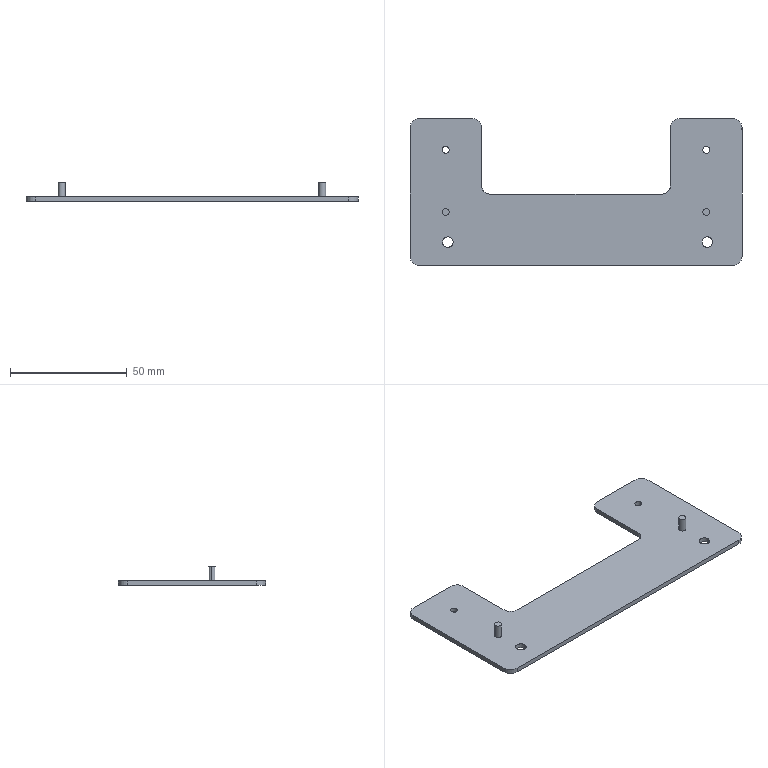Part | NX | features BREP 1 | 1 solid | 32 faces | box 142 x 62.9 x 8 mm | volume 12580 mm3 | cylinder 20 | plane 12 | commonest cylinder face diameters 3 x8 8 x8 4.5 x4
STEP:
#1=CARTESIAN_POINT('',(-233.175,24.9,219.465));
#2=VERTEX_POINT('',#1);
#3=CARTESIAN_POINT('',(-233.175,24.9,225.465));
#4=VERTEX_POINT('',#3);
#5=CARTESIAN_POINT('',(-233.175,24.9,222.465));
#6=DIRECTION('',(0.,0.,1.));
#7=VECTOR('',#6,1000.);
#8=LINE('',#5,#7);
#9=EDGE_CURVE('',#2,#4,#8,.T.);
#10=ORIENTED_EDGE('',*,*,#9,.F.);
#11=CARTESIAN_POINT('',(-236.175,24.9,219.465));
#12=VERTEX_POINT('',#11);
#13=CARTESIAN_POINT('',(-234.675,24.9,219.465));
#14=DIRECTION('',(0.,0.,1.));
#15=DIRECTION('',(1.,0.,0.));
#16=AXIS2_PLACEMENT_3D('',#13,#14,#15);
#17=CIRCLE('',#16,1.5);
#18=EDGE_CURVE('',#2,#12,#17,.T.);
#19=ORIENTED_EDGE('',*,*,#18,.T.);
#20=CARTESIAN_POINT('',(-236.175,24.9,225.465));
#21=VERTEX_POINT('',#20);
#22=CARTESIAN_POINT('',(-236.175,24.9,222.465));
#23=DIRECTION('',(0.,0.,1.));
#24=VECTOR('',#23,1000.);
#25=LINE('',#22,#24);
#26=EDGE_CURVE('',#12,#21,#25,.T.);
#27=ORIENTED_EDGE('',*,*,#26,.T.);
#28=CARTESIAN_POINT('',(-234.675,24.9,225.465));
#29=DIRECTION('',(0.,0.,1.));
#30=DIRECTION('',(1.,0.,0.));
#31=AXIS2_PLACEMENT_3D('',#28,#29,#30);
#32=CIRCLE('',#31,1.5);
#33=EDGE_CURVE('',#4,#21,#32,.T.);
#34=ORIENTED_EDGE('',*,*,#33,.F.);
#35=EDGE_LOOP('',(#10,#19,#27,#34));
#36=FACE_BOUND('',#35,.T.);
#37=CARTESIAN_POINT('',(-234.675,24.9,222.465));
#38=DIRECTION('',(0.,0.,1.));
#39=DIRECTION('',(1.,0.,0.));
#40=AXIS2_PLACEMENT_3D('',#37,#38,#39);
#41=CYLINDRICAL_SURFACE('',#40,1.5);
#42=ADVANCED_FACE('',(#36),#41,.T.);
#43=ORIENTED_EDGE('',*,*,#26,.F.);
#44=CARTESIAN_POINT('',(-234.675,24.9,219.465));
#45=DIRECTION('',(0.,0.,1.));
#46=DIRECTION('',(1.,0.,0.));
#47=AXIS2_PLACEMENT_3D('',#44,#45,#46);
#48=CIRCLE('',#47,1.5);
#49=EDGE_CURVE('',#12,#2,#48,.T.);
#50=ORIENTED_EDGE('',*,*,#49,.T.);
#51=ORIENTED_EDGE('',*,*,#9,.T.);
#52=CARTESIAN_POINT('',(-234.675,24.9,225.465));
#53=DIRECTION('',(0.,0.,1.));
#54=DIRECTION('',(1.,0.,0.));
#55=AXIS2_PLACEMENT_3D('',#52,#53,#54);
#56=CIRCLE('',#55,1.5);
#57=EDGE_CURVE('',#21,#4,#56,.T.);
#58=ORIENTED_EDGE('',*,*,#57,.F.);
#59=EDGE_LOOP('',(#43,#50,#51,#58));
#60=FACE_BOUND('',#59,.T.);
#61=CARTESIAN_POINT('',(-234.675,24.9,222.465));
#62=DIRECTION('',(0.,0.,1.));
#63=DIRECTION('',(1.,0.,0.));
#64=AXIS2_PLACEMENT_3D('',#61,#62,#63);
#65=CYLINDRICAL_SURFACE('',#64,1.5);
#66=ADVANCED_FACE('',(#60),#65,.T.);
#67=ORIENTED_EDGE('',*,*,#33,.T.);
#68=ORIENTED_EDGE('',*,*,#57,.T.);
#69=EDGE_LOOP('',(#67,#68));
#70=FACE_BOUND('',#69,.T.);
#71=CARTESIAN_POINT('',(0.,-0.000000001,225.465));
#72=DIRECTION('',(0.,0.,1.));
#73=DIRECTION('',(1.,0.,0.));
#74=AXIS2_PLACEMENT_3D('',#71,#72,#73);
#75=PLANE('',#74);
#76=ADVANCED_FACE('',(#70),#75,.T.);
#77=CARTESIAN_POINT('',(-245.925,64.9,219.465));
#78=VERTEX_POINT('',#77);
#79=CARTESIAN_POINT('',(-249.925,60.9,219.465));
#80=VERTEX_POINT('',#79);
#81=CARTESIAN_POINT('',(-245.925,60.9,219.465));
#82=DIRECTION('',(0.,0.,1.));
#83=DIRECTION('',(1.,0.,0.));
#84=AXIS2_PLACEMENT_3D('',#81,#82,#83);
#85=CIRCLE('',#84,4.);
#86=EDGE_CURVE('',#78,#80,#85,.T.);
#87=ORIENTED_EDGE('',*,*,#86,.T.);
#88=CARTESIAN_POINT('',(-249.925,6.,219.465));
#89=VERTEX_POINT('',#88);
#90=CARTESIAN_POINT('',(-249.925,33.45,219.465));
#91=DIRECTION('',(0.,1.,0.));
#92=VECTOR('',#91,1000.);
#93=LINE('',#90,#92);
#94=EDGE_CURVE('',#89,#80,#93,.T.);
#95=ORIENTED_EDGE('',*,*,#94,.F.);
#96=CARTESIAN_POINT('',(-245.925,2.,219.465));
#97=VERTEX_POINT('',#96);
#98=CARTESIAN_POINT('',(-245.925,6.,219.465));
#99=DIRECTION('',(0.,0.,1.));
#100=DIRECTION('',(1.,0.,0.));
#101=AXIS2_PLACEMENT_3D('',#98,#99,#100);
#102=CIRCLE('',#101,4.);
#103=EDGE_CURVE('',#89,#97,#102,.T.);
#104=ORIENTED_EDGE('',*,*,#103,.T.);
#105=CARTESIAN_POINT('',(-111.925,2.,219.465));
#106=VERTEX_POINT('',#105);
#107=CARTESIAN_POINT('',(-178.925,2.,219.465));
#108=DIRECTION('',(-1.,0.,0.));
#109=VECTOR('',#108,1000.);
#110=LINE('',#107,#109);
#111=EDGE_CURVE('',#106,#97,#110,.T.);
#112=ORIENTED_EDGE('',*,*,#111,.F.);
#113=CARTESIAN_POINT('',(-107.925,6.,219.465));
#114=VERTEX_POINT('',#113);
#115=CARTESIAN_POINT('',(-111.925,6.,219.465));
#116=DIRECTION('',(0.,0.,1.));
#117=DIRECTION('',(1.,0.,0.));
#118=AXIS2_PLACEMENT_3D('',#115,#116,#117);
#119=CIRCLE('',#118,4.);
#120=EDGE_CURVE('',#106,#114,#119,.T.);
#121=ORIENTED_EDGE('',*,*,#120,.T.);
#122=CARTESIAN_POINT('',(-107.925,60.9,219.465));
#123=VERTEX_POINT('',#122);
#124=CARTESIAN_POINT('',(-107.925,33.45,219.465));
#125=DIRECTION('',(0.,-1.,0.));
#126=VECTOR('',#125,1000.);
#127=LINE('',#124,#126);
#128=EDGE_CURVE('',#123,#114,#127,.T.);
#129=ORIENTED_EDGE('',*,*,#128,.F.);
#130=CARTESIAN_POINT('',(-111.925,64.9,219.465));
#131=VERTEX_POINT('',#130);
#132=CARTESIAN_POINT('',(-111.925,60.9,219.465));
#133=DIRECTION('',(0.,0.,1.));
#134=DIRECTION('',(1.,0.,0.));
#135=AXIS2_PLACEMENT_3D('',#132,#133,#134);
#136=CIRCLE('',#135,4.);
#137=EDGE_CURVE('',#123,#131,#136,.T.);
#138=ORIENTED_EDGE('',*,*,#137,.T.);
#139=CARTESIAN_POINT('',(-134.425,64.9,219.465));
#140=VERTEX_POINT('',#139);
#141=CARTESIAN_POINT('',(-123.175,64.9,219.465));
#142=DIRECTION('',(-1.,0.,0.));
#143=VECTOR('',#142,1000.);
#144=LINE('',#141,#143);
#145=EDGE_CURVE('',#131,#140,#144,.T.);
#146=ORIENTED_EDGE('',*,*,#145,.T.);
#147=CARTESIAN_POINT('',(-138.425,60.9,219.465));
#148=VERTEX_POINT('',#147);
#149=CARTESIAN_POINT('',(-134.425,60.9,219.465));
#150=DIRECTION('',(0.,0.,1.));
#151=DIRECTION('',(1.,0.,0.));
#152=AXIS2_PLACEMENT_3D('',#149,#150,#151);
#153=CIRCLE('',#152,4.);
#154=EDGE_CURVE('',#140,#148,#153,.T.);
#155=ORIENTED_EDGE('',*,*,#154,.T.);
#156=CARTESIAN_POINT('',(-138.425,36.5,219.465));
#157=VERTEX_POINT('',#156);
#158=CARTESIAN_POINT('',(-138.425,48.7,219.465));
#159=DIRECTION('',(0.,1.,0.));
#160=VECTOR('',#159,1000.);
#161=LINE('',#158,#160);
#162=EDGE_CURVE('',#157,#148,#161,.T.);
#163=ORIENTED_EDGE('',*,*,#162,.F.);
#164=CARTESIAN_POINT('',(-142.425,32.5,219.465));
#165=VERTEX_POINT('',#164);
#166=CARTESIAN_POINT('',(-138.425,36.5,219.465));
#167=CARTESIAN_POINT('',(-138.425,36.108,219.465));
#168=CARTESIAN_POINT('',(-138.473,35.716,219.465));
#169=CARTESIAN_POINT('',(-138.569,35.332,219.465));
#170=CARTESIAN_POINT('',(-138.853,34.595,219.465));
#171=CARTESIAN_POINT('',(-139.307,33.949,219.465));
#172=CARTESIAN_POINT('',(-139.572,33.655,219.465));
#173=CARTESIAN_POINT('',(-140.169,33.139,219.465));
#174=CARTESIAN_POINT('',(-140.874,32.782,219.465));
#175=CARTESIAN_POINT('',(-141.246,32.647,219.465));
#176=CARTESIAN_POINT('',(-141.711,32.542,219.465));
#177=CARTESIAN_POINT('',(-142.182,32.506,219.465));
#178=CARTESIAN_POINT('',(-142.263,32.502,219.465));
#179=CARTESIAN_POINT('',(-142.344,32.5,219.465));
#180=CARTESIAN_POINT('',(-142.425,32.5,219.465));
#181=B_SPLINE_CURVE_WITH_KNOTS('',5,(#166,#167,#168,#169,#170,#171,#172,#173,#174,#175,#176,#177,#178,#179,#180),.UNSPECIFIED.,.F.,.F.,(6,3,3,3,6),(0.,0.3119,0.6238,0.9356,1.),.UNSPECIFIED.);
#182=EDGE_CURVE('',#157,#165,#181,.T.);
#183=ORIENTED_EDGE('',*,*,#182,.T.);
#184=CARTESIAN_POINT('',(-215.425,32.5,219.465));
#185=VERTEX_POINT('',#184);
#186=CARTESIAN_POINT('',(-178.925,32.5,219.465));
#187=DIRECTION('',(1.,0.,0.));
#188=VECTOR('',#187,1000.);
#189=LINE('',#186,#188);
#190=EDGE_CURVE('',#185,#165,#189,.T.);
#191=ORIENTED_EDGE('',*,*,#190,.F.);
#192=CARTESIAN_POINT('',(-219.425,36.5,219.465));
#193=VERTEX_POINT('',#192);
#194=CARTESIAN_POINT('',(-215.425,32.5,219.465));
#195=CARTESIAN_POINT('',(-215.817,32.5,219.465));
#196=CARTESIAN_POINT('',(-216.209,32.548,219.465));
#197=CARTESIAN_POINT('',(-216.593,32.644,219.465));
#198=CARTESIAN_POINT('',(-217.33,32.928,219.465));
#199=CARTESIAN_POINT('',(-217.976,33.382,219.465));
#200=CARTESIAN_POINT('',(-218.27,33.647,219.465));
#201=CARTESIAN_POINT('',(-218.786,34.244,219.465));
#202=CARTESIAN_POINT('',(-219.143,34.949,219.465));
#203=CARTESIAN_POINT('',(-219.278,35.321,219.465));
#204=CARTESIAN_POINT('',(-219.383,35.786,219.465));
#205=CARTESIAN_POINT('',(-219.419,36.257,219.465));
#206=CARTESIAN_POINT('',(-219.423,36.338,219.465));
#207=CARTESIAN_POINT('',(-219.425,36.419,219.465));
#208=CARTESIAN_POINT('',(-219.425,36.5,219.465));
#209=B_SPLINE_CURVE_WITH_KNOTS('',5,(#194,#195,#196,#197,#198,#199,#200,#201,#202,#203,#204,#205,#206,#207,#208),.UNSPECIFIED.,.F.,.F.,(6,3,3,3,6),(0.,0.3119,0.6238,0.9356,1.),.UNSPECIFIED.);
#210=EDGE_CURVE('',#185,#193,#209,.T.);
#211=ORIENTED_EDGE('',*,*,#210,.T.);
#212=CARTESIAN_POINT('',(-219.425,60.9,219.465));
#213=VERTEX_POINT('',#212);
#214=CARTESIAN_POINT('',(-219.425,48.7,219.465));
#215=DIRECTION('',(0.,-1.,0.));
#216=VECTOR('',#215,1000.);
#217=LINE('',#214,#216);
#218=EDGE_CURVE('',#213,#193,#217,.T.);
#219=ORIENTED_EDGE('',*,*,#218,.F.);
#220=CARTESIAN_POINT('',(-223.425,64.9,219.465));
#221=VERTEX_POINT('',#220);
#222=CARTESIAN_POINT('',(-223.425,60.9,219.465));
#223=DIRECTION('',(0.,0.,1.));
#224=DIRECTION('',(1.,0.,0.));
#225=AXIS2_PLACEMENT_3D('',#222,#223,#224);
#226=CIRCLE('',#225,4.);
#227=EDGE_CURVE('',#213,#221,#226,.T.);
#228=ORIENTED_EDGE('',*,*,#227,.T.);
#229=CARTESIAN_POINT('',(-234.675,64.9,219.465));
#230=DIRECTION('',(-1.,0.,0.));
#231=VECTOR('',#230,1000.);
#232=LINE('',#229,#231);
#233=EDGE_CURVE('',#221,#78,#232,.T.);
#234=ORIENTED_EDGE('',*,*,#233,.T.);
#235=EDGE_LOOP('',(#87,#95,#104,#112,#121,#129,#138,#146,#155,#163,#183,#191,#211,#219,#228,#234));
#236=FACE_BOUND('',#235,.T.);
#237=CARTESIAN_POINT('',(-121.675,24.9,219.465));
#238=VERTEX_POINT('',#237);
#239=CARTESIAN_POINT('',(-124.675,24.9,219.465));
#240=VERTEX_POINT('',#239);
#241=CARTESIAN_POINT('',(-123.175,24.9,219.465));
#242=DIRECTION('',(0.,0.,1.));
#243=DIRECTION('',(1.,0.,0.));
#244=AXIS2_PLACEMENT_3D('',#241,#242,#243);
#245=CIRCLE('',#244,1.5);
#246=EDGE_CURVE('',#238,#240,#245,.T.);
#247=ORIENTED_EDGE('',*,*,#246,.F.);
#248=CARTESIAN_POINT('',(-123.175,24.9,219.465));
#249=DIRECTION('',(0.,0.,1.));
#250=DIRECTION('',(1.,0.,0.));
#251=AXIS2_PLACEMENT_3D('',#248,#249,#250);
#252=CIRCLE('',#251,1.5);
#253=EDGE_CURVE('',#240,#238,#252,.T.);
#254=ORIENTED_EDGE('',*,*,#253,.F.);
#255=EDGE_LOOP('',(#247,#254));
#256=FACE_BOUND('',#255,.T.);
#257=ORIENTED_EDGE('',*,*,#18,.F.);
#258=ORIENTED_EDGE('',*,*,#49,.F.);
#259=EDGE_LOOP('',(#257,#258));
#260=FACE_BOUND('',#259,.T.);
#261=CARTESIAN_POINT('',(-236.,12.,219.465));
#262=VERTEX_POINT('',#261);
#263=CARTESIAN_POINT('',(-231.5,12.,219.465));
#264=VERTEX_POINT('',#263);
#265=CARTESIAN_POINT('',(-236.,12.,219.465));
#266=CARTESIAN_POINT('',(-236.,12.22,219.465));
#267=CARTESIAN_POINT('',(-235.973,12.441,219.465));
#268=CARTESIAN_POINT('',(-235.919,12.657,219.465));
#269=CARTESIAN_POINT('',(-235.759,13.071,219.465));
#270=CARTESIAN_POINT('',(-235.504,13.435,219.465));
#271=CARTESIAN_POINT('',(-235.355,13.6,219.465));
#272=CARTESIAN_POINT('',(-235.019,13.891,219.465));
#273=CARTESIAN_POINT('',(-234.623,14.092,219.465));
#274=CARTESIAN_POINT('',(-234.413,14.167,219.465));
#275=CARTESIAN_POINT('',(-233.98,14.265,219.465));
#276=CARTESIAN_POINT('',(-233.536,14.256,219.465));
#277=CARTESIAN_POINT('',(-233.315,14.224,219.465));
#278=CARTESIAN_POINT('',(-232.887,14.107,219.465));
#279=CARTESIAN_POINT('',(-232.499,13.89,219.465));
#280=CARTESIAN_POINT('',(-232.32,13.758,219.465));
#281=CARTESIAN_POINT('',(-231.997,13.453,219.465));
#282=CARTESIAN_POINT('',(-231.757,13.079,219.465));
#283=CARTESIAN_POINT('',(-231.661,12.878,219.465));
#284=CARTESIAN_POINT('',(-231.561,12.581,219.465));
#285=CARTESIAN_POINT('',(-231.514,12.273,219.465));
#286=CARTESIAN_POINT('',(-231.505,12.182,219.465));
#287=CARTESIAN_POINT('',(-231.5,12.091,219.465));
#288=CARTESIAN_POINT('',(-231.5,12.,219.465));
#289=B_SPLINE_CURVE_WITH_KNOTS('',5,(#265,#266,#267,#268,#269,#270,#271,#272,#273,#274,#275,#276,#277,#278,#279,#280,#281,#282,#283,#284,#285,#286,#287,#288),.UNSPECIFIED.,.F.,.F.,(6,3,3,3,3,3,3,6),(0.,0.156,0.3119,0.4679,0.6238,0.7798,0.9357,1.),.UNSPECIFIED.);
#290=EDGE_CURVE('',#262,#264,#289,.T.);
#291=ORIENTED_EDGE('',*,*,#290,.T.);
#292=CARTESIAN_POINT('',(-231.5,12.,219.465));
#293=CARTESIAN_POINT('',(-231.5,11.78,219.465));
#294=CARTESIAN_POINT('',(-231.527,11.559,219.465));
#295=CARTESIAN_POINT('',(-231.581,11.343,219.465));
#296=CARTESIAN_POINT('',(-231.741,10.929,219.465));
#297=CARTESIAN_POINT('',(-231.996,10.565,219.465));
#298=CARTESIAN_POINT('',(-232.145,10.4,219.465));
#299=CARTESIAN_POINT('',(-232.481,10.109,219.465));
#300=CARTESIAN_POINT('',(-232.877,9.908,219.465));
#301=CARTESIAN_POINT('',(-233.087,9.833,219.465));
#302=CARTESIAN_POINT('',(-233.52,9.735,219.465));
#303=CARTESIAN_POINT('',(-233.964,9.744,219.465));
#304=CARTESIAN_POINT('',(-234.185,9.776,219.465));
#305=CARTESIAN_POINT('',(-234.613,9.893,219.465));
#306=CARTESIAN_POINT('',(-235.001,10.11,219.465));
#307=CARTESIAN_POINT('',(-235.18,10.242,219.465));
#308=CARTESIAN_POINT('',(-235.503,10.547,219.465));
#309=CARTESIAN_POINT('',(-235.743,10.921,219.465));
#310=CARTESIAN_POINT('',(-235.839,11.122,219.465));
#311=CARTESIAN_POINT('',(-235.939,11.419,219.465));
#312=CARTESIAN_POINT('',(-235.986,11.727,219.465));
#313=CARTESIAN_POINT('',(-235.995,11.818,219.465));
#314=CARTESIAN_POINT('',(-236.,11.909,219.465));
#315=CARTESIAN_POINT('',(-236.,12.,219.465));
#316=B_SPLINE_CURVE_WITH_KNOTS('',5,(#292,#293,#294,#295,#296,#297,#298,#299,#300,#301,#302,#303,#304,#305,#306,#307,#308,#309,#310,#311,#312,#313,#314,#315),.UNSPECIFIED.,.F.,.F.,(6,3,3,3,3,3,3,6),(0.,0.156,0.3119,0.4679,0.6238,0.7798,0.9357,1.),.UNSPECIFIED.);
#317=EDGE_CURVE('',#264,#262,#316,.T.);
#318=ORIENTED_EDGE('',*,*,#317,.T.);
#319=EDGE_LOOP('',(#291,#318));
#320=FACE_BOUND('',#319,.T.);
#321=CARTESIAN_POINT('',(-125.,12.,219.465));
#322=VERTEX_POINT('',#321);
#323=CARTESIAN_POINT('',(-120.5,12.,219.465));
#324=VERTEX_POINT('',#323);
#325=CARTESIAN_POINT('',(-125.,12.,219.465));
#326=CARTESIAN_POINT('',(-125.,12.22,219.465));
#327=CARTESIAN_POINT('',(-124.973,12.441,219.465));
#328=CARTESIAN_POINT('',(-124.919,12.657,219.465));
#329=CARTESIAN_POINT('',(-124.759,13.071,219.465));
#330=CARTESIAN_POINT('',(-124.504,13.435,219.465));
#331=CARTESIAN_POINT('',(-124.355,13.6,219.465));
#332=CARTESIAN_POINT('',(-124.019,13.891,219.465));
#333=CARTESIAN_POINT('',(-123.623,14.092,219.465));
#334=CARTESIAN_POINT('',(-123.413,14.167,219.465));
#335=CARTESIAN_POINT('',(-122.98,14.265,219.465));
#336=CARTESIAN_POINT('',(-122.536,14.256,219.465));
#337=CARTESIAN_POINT('',(-122.315,14.224,219.465));
#338=CARTESIAN_POINT('',(-121.887,14.107,219.465));
#339=CARTESIAN_POINT('',(-121.499,13.89,219.465));
#340=CARTESIAN_POINT('',(-121.32,13.758,219.465));
#341=CARTESIAN_POINT('',(-120.997,13.453,219.465));
#342=CARTESIAN_POINT('',(-120.757,13.079,219.465));
#343=CARTESIAN_POINT('',(-120.661,12.878,219.465));
#344=CARTESIAN_POINT('',(-120.561,12.581,219.465));
#345=CARTESIAN_POINT('',(-120.514,12.273,219.465));
#346=CARTESIAN_POINT('',(-120.505,12.182,219.465));
#347=CARTESIAN_POINT('',(-120.5,12.091,219.465));
#348=CARTESIAN_POINT('',(-120.5,12.,219.465));
#349=B_SPLINE_CURVE_WITH_KNOTS('',5,(#325,#326,#327,#328,#329,#330,#331,#332,#333,#334,#335,#336,#337,#338,#339,#340,#341,#342,#343,#344,#345,#346,#347,#348),.UNSPECIFIED.,.F.,.F.,(6,3,3,3,3,3,3,6),(0.,0.156,0.3119,0.4679,0.6238,0.7798,0.9357,1.),.UNSPECIFIED.);
#350=EDGE_CURVE('',#322,#324,#349,.T.);
#351=ORIENTED_EDGE('',*,*,#350,.T.);
#352=CARTESIAN_POINT('',(-120.5,12.,219.465));
#353=CARTESIAN_POINT('',(-120.5,11.78,219.465));
#354=CARTESIAN_POINT('',(-120.527,11.559,219.465));
#355=CARTESIAN_POINT('',(-120.581,11.343,219.465));
#356=CARTESIAN_POINT('',(-120.741,10.929,219.465));
#357=CARTESIAN_POINT('',(-120.996,10.565,219.465));
#358=CARTESIAN_POINT('',(-121.145,10.4,219.465));
#359=CARTESIAN_POINT('',(-121.481,10.109,219.465));
#360=CARTESIAN_POINT('',(-121.877,9.908,219.465));
#361=CARTESIAN_POINT('',(-122.087,9.833,219.465));
#362=CARTESIAN_POINT('',(-122.52,9.735,219.465));
#363=CARTESIAN_POINT('',(-122.964,9.744,219.465));
#364=CARTESIAN_POINT('',(-123.185,9.776,219.465));
#365=CARTESIAN_POINT('',(-123.613,9.893,219.465));
#366=CARTESIAN_POINT('',(-124.001,10.11,219.465));
#367=CARTESIAN_POINT('',(-124.18,10.242,219.465));
#368=CARTESIAN_POINT('',(-124.503,10.547,219.465));
#369=CARTESIAN_POINT('',(-124.743,10.921,219.465));
#370=CARTESIAN_POINT('',(-124.839,11.122,219.465));
#371=CARTESIAN_POINT('',(-124.939,11.419,219.465));
#372=CARTESIAN_POINT('',(-124.986,11.727,219.465));
#373=CARTESIAN_POINT('',(-124.995,11.818,219.465));
#374=CARTESIAN_POINT('',(-125.,11.909,219.465));
#375=CARTESIAN_POINT('',(-125.,12.,219.465));
#376=B_SPLINE_CURVE_WITH_KNOTS('',5,(#352,#353,#354,#355,#356,#357,#358,#359,#360,#361,#362,#363,#364,#365,#366,#367,#368,#369,#370,#371,#372,#373,#374,#375),.UNSPECIFIED.,.F.,.F.,(6,3,3,3,3,3,3,6),(0.,0.156,0.3119,0.4679,0.6238,0.7798,0.9357,1.),.UNSPECIFIED.);
#377=EDGE_CURVE('',#324,#322,#376,.T.);
#378=ORIENTED_EDGE('',*,*,#377,.T.);
#379=EDGE_LOOP('',(#351,#378));
#380=FACE_BOUND('',#379,.T.);
#381=CARTESIAN_POINT('',(-236.175,51.5,219.465));
#382=VERTEX_POINT('',#381);
#383=CARTESIAN_POINT('',(-233.175,51.5,219.465));
#384=VERTEX_POINT('',#383);
#385=CARTESIAN_POINT('',(-236.175,51.5,219.465));
#386=CARTESIAN_POINT('',(-236.175,51.68,219.465));
#387=CARTESIAN_POINT('',(-236.148,51.86,219.465));
#388=CARTESIAN_POINT('',(-236.094,52.035,219.465));
#389=CARTESIAN_POINT('',(-235.935,52.362,219.465));
#390=CARTESIAN_POINT('',(-235.687,52.629,219.465));
#391=CARTESIAN_POINT('',(-235.544,52.742,219.465));
#392=CARTESIAN_POINT('',(-235.228,52.923,219.465));
#393=CARTESIAN_POINT('',(-234.873,53.003,219.465));
#394=CARTESIAN_POINT('',(-234.691,53.016,219.465));
#395=CARTESIAN_POINT('',(-234.328,52.987,219.465));
#396=CARTESIAN_POINT('',(-233.99,52.853,219.465));
#397=CARTESIAN_POINT('',(-233.832,52.76,219.465));
#398=CARTESIAN_POINT('',(-233.549,52.531,219.465));
#399=CARTESIAN_POINT('',(-233.346,52.23,219.465));
#400=CARTESIAN_POINT('',(-233.268,52.064,219.465));
#401=CARTESIAN_POINT('',(-233.203,51.849,219.465));
#402=CARTESIAN_POINT('',(-233.18,51.627,219.465));
#403=CARTESIAN_POINT('',(-233.177,51.585,219.465));
#404=CARTESIAN_POINT('',(-233.175,51.542,219.465));
#405=CARTESIAN_POINT('',(-233.175,51.5,219.465));
#406=B_SPLINE_CURVE_WITH_KNOTS('',5,(#385,#386,#387,#388,#389,#390,#391,#392,#393,#394,#395,#396,#397,#398,#399,#400,#401,#402,#403,#404,#405),.UNSPECIFIED.,.F.,.F.,(6,3,3,3,3,3,6),(0.,0.191,0.382,0.573,0.764,0.9549,1.),.UNSPECIFIED.);
#407=EDGE_CURVE('',#382,#384,#406,.T.);
#408=ORIENTED_EDGE('',*,*,#407,.T.);
#409=CARTESIAN_POINT('',(-233.175,51.5,219.465));
#410=CARTESIAN_POINT('',(-233.175,51.32,219.465));
#411=CARTESIAN_POINT('',(-233.202,51.14,219.465));
#412=CARTESIAN_POINT('',(-233.256,50.965,219.465));
#413=CARTESIAN_POINT('',(-233.415,50.638,219.465));
#414=CARTESIAN_POINT('',(-233.663,50.371,219.465));
#415=CARTESIAN_POINT('',(-233.806,50.258,219.465));
#416=CARTESIAN_POINT('',(-234.122,50.077,219.465));
#417=CARTESIAN_POINT('',(-234.477,49.997,219.465));
#418=CARTESIAN_POINT('',(-234.659,49.984,219.465));
#419=CARTESIAN_POINT('',(-235.022,50.013,219.465));
#420=CARTESIAN_POINT('',(-235.36,50.147,219.465));
#421=CARTESIAN_POINT('',(-235.518,50.24,219.465));
#422=CARTESIAN_POINT('',(-235.801,50.469,219.465));
#423=CARTESIAN_POINT('',(-236.004,50.77,219.465));
#424=CARTESIAN_POINT('',(-236.082,50.936,219.465));
#425=CARTESIAN_POINT('',(-236.147,51.151,219.465));
#426=CARTESIAN_POINT('',(-236.17,51.373,219.465));
#427=CARTESIAN_POINT('',(-236.173,51.415,219.465));
#428=CARTESIAN_POINT('',(-236.175,51.458,219.465));
#429=CARTESIAN_POINT('',(-236.175,51.5,219.465));
#430=B_SPLINE_CURVE_WITH_KNOTS('',5,(#409,#410,#411,#412,#413,#414,#415,#416,#417,#418,#419,#420,#421,#422,#423,#424,#425,#426,#427,#428,#429),.UNSPECIFIED.,.F.,.F.,(6,3,3,3,3,3,6),(0.,0.191,0.382,0.573,0.764,0.9549,1.),.UNSPECIFIED.);
#431=EDGE_CURVE('',#384,#382,#430,.T.);
#432=ORIENTED_EDGE('',*,*,#431,.T.);
#433=EDGE_LOOP('',(#408,#432));
#434=FACE_BOUND('',#433,.T.);
#435=CARTESIAN_POINT('',(-124.675,51.5,219.465));
#436=VERTEX_POINT('',#435);
#437=CARTESIAN_POINT('',(-121.675,51.5,219.465));
#438=VERTEX_POINT('',#437);
#439=CARTESIAN_POINT('',(-124.675,51.5,219.465));
#440=CARTESIAN_POINT('',(-124.675,51.68,219.465));
#441=CARTESIAN_POINT('',(-124.648,51.86,219.465));
#442=CARTESIAN_POINT('',(-124.594,52.035,219.465));
#443=CARTESIAN_POINT('',(-124.435,52.362,219.465));
#444=CARTESIAN_POINT('',(-124.187,52.629,219.465));
#445=CARTESIAN_POINT('',(-124.044,52.742,219.465));
#446=CARTESIAN_POINT('',(-123.728,52.923,219.465));
#447=CARTESIAN_POINT('',(-123.373,53.003,219.465));
#448=CARTESIAN_POINT('',(-123.191,53.016,219.465));
#449=CARTESIAN_POINT('',(-122.828,52.987,219.465));
#450=CARTESIAN_POINT('',(-122.49,52.853,219.465));
#451=CARTESIAN_POINT('',(-122.332,52.76,219.465));
#452=CARTESIAN_POINT('',(-122.049,52.531,219.465));
#453=CARTESIAN_POINT('',(-121.846,52.229,219.465));
#454=CARTESIAN_POINT('',(-121.768,52.064,219.465));
#455=CARTESIAN_POINT('',(-121.703,51.849,219.465));
#456=CARTESIAN_POINT('',(-121.68,51.627,219.465));
#457=CARTESIAN_POINT('',(-121.677,51.585,219.465));
#458=CARTESIAN_POINT('',(-121.675,51.542,219.465));
#459=CARTESIAN_POINT('',(-121.675,51.5,219.465));
#460=B_SPLINE_CURVE_WITH_KNOTS('',5,(#439,#440,#441,#442,#443,#444,#445,#446,#447,#448,#449,#450,#451,#452,#453,#454,#455,#456,#457,#458,#459),.UNSPECIFIED.,.F.,.F.,(6,3,3,3,3,3,6),(0.,0.191,0.382,0.573,0.764,0.955,1.),.UNSPECIFIED.);
#461=EDGE_CURVE('',#436,#438,#460,.T.);
#462=ORIENTED_EDGE('',*,*,#461,.T.);
#463=CARTESIAN_POINT('',(-121.675,51.5,219.465));
#464=CARTESIAN_POINT('',(-121.675,51.32,219.465));
#465=CARTESIAN_POINT('',(-121.702,51.14,219.465));
#466=CARTESIAN_POINT('',(-121.756,50.965,219.465));
#467=CARTESIAN_POINT('',(-121.915,50.638,219.465));
#468=CARTESIAN_POINT('',(-122.163,50.371,219.465));
#469=CARTESIAN_POINT('',(-122.306,50.258,219.465));
#470=CARTESIAN_POINT('',(-122.622,50.077,219.465));
#471=CARTESIAN_POINT('',(-122.977,49.997,219.465));
#472=CARTESIAN_POINT('',(-123.159,49.984,219.465));
#473=CARTESIAN_POINT('',(-123.522,50.013,219.465));
#474=CARTESIAN_POINT('',(-123.86,50.147,219.465));
#475=CARTESIAN_POINT('',(-124.018,50.24,219.465));
#476=CARTESIAN_POINT('',(-124.301,50.469,219.465));
#477=CARTESIAN_POINT('',(-124.504,50.771,219.465));
#478=CARTESIAN_POINT('',(-124.582,50.936,219.465));
#479=CARTESIAN_POINT('',(-124.647,51.151,219.465));
#480=CARTESIAN_POINT('',(-124.67,51.373,219.465));
#481=CARTESIAN_POINT('',(-124.673,51.415,219.465));
#482=CARTESIAN_POINT('',(-124.675,51.458,219.465));
#483=CARTESIAN_POINT('',(-124.675,51.5,219.465));
#484=B_SPLINE_CURVE_WITH_KNOTS('',5,(#463,#464,#465,#466,#467,#468,#469,#470,#471,#472,#473,#474,#475,#476,#477,#478,#479,#480,#481,#482,#483),.UNSPECIFIED.,.F.,.F.,(6,3,3,3,3,3,6),(0.,0.191,0.382,0.573,0.764,0.955,1.),.UNSPECIFIED.);
#485=EDGE_CURVE('',#438,#436,#484,.T.);
#486=ORIENTED_EDGE('',*,*,#485,.T.);
#487=EDGE_LOOP('',(#462,#486));
#488=FACE_BOUND('',#487,.T.);
#489=CARTESIAN_POINT('',(-357.85,212.,219.465));
#490=DIRECTION('',(0.,0.,1.));
#491=DIRECTION('',(0.,1.,0.));
#492=AXIS2_PLACEMENT_3D('',#489,#490,#491);
#493=PLANE('',#492);
#494=ADVANCED_FACE('',(#236,#256,#260,#320,#380,#434,#488),#493,.T.);
#495=CARTESIAN_POINT('',(-124.675,51.5,217.465));
#496=VERTEX_POINT('',#495);
#497=CARTESIAN_POINT('',(-124.675,51.5,217.465));
#498=DIRECTION('',(0.,0.,-1.));
#499=VECTOR('',#498,1000.);
#500=LINE('',#497,#499);
#501=EDGE_CURVE('',#436,#496,#500,.T.);
#502=ORIENTED_EDGE('',*,*,#501,.F.);
#503=ORIENTED_EDGE('',*,*,#485,.F.);
#504=CARTESIAN_POINT('',(-121.675,51.5,217.465));
#505=VERTEX_POINT('',#504);
#506=CARTESIAN_POINT('',(-121.675,51.5,217.465));
#507=DIRECTION('',(0.,0.,1.));
#508=VECTOR('',#507,1000.);
#509=LINE('',#506,#508);
#510=EDGE_CURVE('',#505,#438,#509,.T.);
#511=ORIENTED_EDGE('',*,*,#510,.F.);
#512=CARTESIAN_POINT('',(-123.175,51.5,217.465));
#513=DIRECTION('',(0.,0.,1.));
#514=DIRECTION('',(1.,0.,0.));
#515=AXIS2_PLACEMENT_3D('',#512,#513,#514);
#516=CIRCLE('',#515,1.5);
#517=EDGE_CURVE('',#496,#505,#516,.T.);
#518=ORIENTED_EDGE('',*,*,#517,.F.);
#519=EDGE_LOOP('',(#502,#503,#511,#518));
#520=FACE_BOUND('',#519,.T.);
#521=CARTESIAN_POINT('',(-123.175,51.5,217.465));
#522=DIRECTION('',(0.,0.,1.));
#523=DIRECTION('',(-1.,0.,0.));
#524=AXIS2_PLACEMENT_3D('',#521,#522,#523);
#525=CYLINDRICAL_SURFACE('',#524,1.5);
#526=ADVANCED_FACE('',(#520),#525,.F.);
#527=ORIENTED_EDGE('',*,*,#510,.T.);
#528=ORIENTED_EDGE('',*,*,#461,.F.);
#529=ORIENTED_EDGE('',*,*,#501,.T.);
#530=CARTESIAN_POINT('',(-123.175,51.5,217.465));
#531=DIRECTION('',(0.,0.,1.));
#532=DIRECTION('',(1.,0.,0.));
#533=AXIS2_PLACEMENT_3D('',#530,#531,#532);
#534=CIRCLE('',#533,1.5);
#535=EDGE_CURVE('',#505,#496,#534,.T.);
#536=ORIENTED_EDGE('',*,*,#535,.F.);
#537=EDGE_LOOP('',(#527,#528,#529,#536));
#538=FACE_BOUND('',#537,.T.);
#539=CARTESIAN_POINT('',(-123.175,51.5,217.465));
#540=DIRECTION('',(0.,0.,1.));
#541=DIRECTION('',(1.,0.,0.));
#542=AXIS2_PLACEMENT_3D('',#539,#540,#541);
#543=CYLINDRICAL_SURFACE('',#542,1.5);
#544=ADVANCED_FACE('',(#538),#543,.F.);
#545=CARTESIAN_POINT('',(-125.,12.,217.465));
#546=VERTEX_POINT('',#545);
#547=CARTESIAN_POINT('',(-125.,12.,210.465));
#548=DIRECTION('',(0.,0.,1.));
#549=VECTOR('',#548,1000.);
#550=LINE('',#547,#549);
#551=EDGE_CURVE('',#546,#322,#550,.T.);
#552=ORIENTED_EDGE('',*,*,#551,.T.);
#553=ORIENTED_EDGE('',*,*,#377,.F.);
#554=CARTESIAN_POINT('',(-120.5,12.,217.465));
#555=VERTEX_POINT('',#554);
#556=CARTESIAN_POINT('',(-120.5,12.,210.465));
#557=DIRECTION('',(0.,0.,-1.));
#558=VECTOR('',#557,1000.);
#559=LINE('',#556,#558);
#560=EDGE_CURVE('',#324,#555,#559,.T.);
#561=ORIENTED_EDGE('',*,*,#560,.T.);
#562=CARTESIAN_POINT('',(-122.75,12.,217.465));
#563=DIRECTION('',(0.,0.,1.));
#564=DIRECTION('',(1.,0.,0.));
#565=AXIS2_PLACEMENT_3D('',#562,#563,#564);
#566=CIRCLE('',#565,2.25);
#567=EDGE_CURVE('',#546,#555,#566,.T.);
#568=ORIENTED_EDGE('',*,*,#567,.F.);
#569=EDGE_LOOP('',(#552,#553,#561,#568));
#570=FACE_BOUND('',#569,.T.);
#571=CARTESIAN_POINT('',(-122.75,12.,210.465));
#572=DIRECTION('',(0.,0.,1.));
#573=DIRECTION('',(-1.,0.,0.));
#574=AXIS2_PLACEMENT_3D('',#571,#572,#573);
#575=CYLINDRICAL_SURFACE('',#574,2.25);
#576=ADVANCED_FACE('',(#570),#575,.F.);
#577=ORIENTED_EDGE('',*,*,#560,.F.);
#578=ORIENTED_EDGE('',*,*,#350,.F.);
#579=ORIENTED_EDGE('',*,*,#551,.F.);
#580=CARTESIAN_POINT('',(-122.75,12.,217.465));
#581=DIRECTION('',(0.,0.,1.));
#582=DIRECTION('',(1.,0.,0.));
#583=AXIS2_PLACEMENT_3D('',#580,#581,#582);
#584=CIRCLE('',#583,2.25);
#585=EDGE_CURVE('',#555,#546,#584,.T.);
#586=ORIENTED_EDGE('',*,*,#585,.F.);
#587=EDGE_LOOP('',(#577,#578,#579,#586));
#588=FACE_BOUND('',#587,.T.);
#589=CARTESIAN_POINT('',(-122.75,12.,210.465));
#590=DIRECTION('',(0.,0.,1.));
#591=DIRECTION('',(1.,0.,0.));
#592=AXIS2_PLACEMENT_3D('',#589,#590,#591);
#593=CYLINDRICAL_SURFACE('',#592,2.25);
#594=ADVANCED_FACE('',(#588),#593,.F.);
#595=CARTESIAN_POINT('',(-236.,12.,217.465));
#596=VERTEX_POINT('',#595);
#597=CARTESIAN_POINT('',(-236.,12.,210.465));
#598=DIRECTION('',(0.,0.,1.));
#599=VECTOR('',#598,1000.);
#600=LINE('',#597,#599);
#601=EDGE_CURVE('',#596,#262,#600,.T.);
#602=ORIENTED_EDGE('',*,*,#601,.T.);
#603=ORIENTED_EDGE('',*,*,#317,.F.);
#604=CARTESIAN_POINT('',(-231.5,12.,217.465));
#605=VERTEX_POINT('',#604);
#606=CARTESIAN_POINT('',(-231.5,12.,210.465));
#607=DIRECTION('',(0.,0.,-1.));
#608=VECTOR('',#607,1000.);
#609=LINE('',#606,#608);
#610=EDGE_CURVE('',#264,#605,#609,.T.);
#611=ORIENTED_EDGE('',*,*,#610,.T.);
#612=CARTESIAN_POINT('',(-233.75,12.,217.465));
#613=DIRECTION('',(0.,0.,1.));
#614=DIRECTION('',(1.,0.,0.));
#615=AXIS2_PLACEMENT_3D('',#612,#613,#614);
#616=CIRCLE('',#615,2.25);
#617=EDGE_CURVE('',#596,#605,#616,.T.);
#618=ORIENTED_EDGE('',*,*,#617,.F.);
#619=EDGE_LOOP('',(#602,#603,#611,#618));
#620=FACE_BOUND('',#619,.T.);
#621=CARTESIAN_POINT('',(-233.75,12.,210.465));
#622=DIRECTION('',(0.,0.,1.));
#623=DIRECTION('',(-1.,0.,0.));
#624=AXIS2_PLACEMENT_3D('',#621,#622,#623);
#625=CYLINDRICAL_SURFACE('',#624,2.25);
#626=ADVANCED_FACE('',(#620),#625,.F.);
#627=ORIENTED_EDGE('',*,*,#610,.F.);
#628=ORIENTED_EDGE('',*,*,#290,.F.);
#629=ORIENTED_EDGE('',*,*,#601,.F.);
#630=CARTESIAN_POINT('',(-233.75,12.,217.465));
#631=DIRECTION('',(0.,0.,1.));
#632=DIRECTION('',(1.,0.,0.));
#633=AXIS2_PLACEMENT_3D('',#630,#631,#632);
#634=CIRCLE('',#633,2.25);
#635=EDGE_CURVE('',#605,#596,#634,.T.);
#636=ORIENTED_EDGE('',*,*,#635,.F.);
#637=EDGE_LOOP('',(#627,#628,#629,#636));
#638=FACE_BOUND('',#637,.T.);
#639=CARTESIAN_POINT('',(-233.75,12.,210.465));
#640=DIRECTION('',(0.,0.,1.));
#641=DIRECTION('',(1.,0.,0.));
#642=AXIS2_PLACEMENT_3D('',#639,#640,#641);
#643=CYLINDRICAL_SURFACE('',#642,2.25);
#644=ADVANCED_FACE('',(#638),#643,.F.);
#645=CARTESIAN_POINT('',(-245.925,64.9,217.465));
#646=VERTEX_POINT('',#645);
#647=CARTESIAN_POINT('',(-245.925,64.9,218.465));
#648=DIRECTION('',(0.,0.,-1.));
#649=VECTOR('',#648,1000.);
#650=LINE('',#647,#649);
#651=EDGE_CURVE('',#78,#646,#650,.T.);
#652=ORIENTED_EDGE('',*,*,#651,.F.);
#653=ORIENTED_EDGE('',*,*,#233,.F.);
#654=CARTESIAN_POINT('',(-223.425,64.9,217.465));
#655=VERTEX_POINT('',#654);
#656=CARTESIAN_POINT('',(-223.425,64.9,218.465));
#657=DIRECTION('',(0.,0.,1.));
#658=VECTOR('',#657,1000.);
#659=LINE('',#656,#658);
#660=EDGE_CURVE('',#655,#221,#659,.T.);
#661=ORIENTED_EDGE('',*,*,#660,.F.);
#662=CARTESIAN_POINT('',(-234.675,64.9,217.465));
#663=DIRECTION('',(1.,0.,0.));
#664=VECTOR('',#663,1000.);
#665=LINE('',#662,#664);
#666=EDGE_CURVE('',#646,#655,#665,.T.);
#667=ORIENTED_EDGE('',*,*,#666,.F.);
#668=EDGE_LOOP('',(#652,#653,#661,#667));
#669=FACE_BOUND('',#668,.T.);
#670=CARTESIAN_POINT('',(-178.925,64.9,217.465));
#671=DIRECTION('',(0.,1.,0.));
#672=DIRECTION('',(-1.,0.,0.));
#673=AXIS2_PLACEMENT_3D('',#670,#671,#672);
#674=PLANE('',#673);
#675=ADVANCED_FACE('',(#669),#674,.T.);
#676=ORIENTED_EDGE('',*,*,#660,.T.);
#677=ORIENTED_EDGE('',*,*,#227,.F.);
#678=CARTESIAN_POINT('',(-219.425,60.9,217.465));
#679=VERTEX_POINT('',#678);
#680=CARTESIAN_POINT('',(-219.425,60.9,217.465));
#681=DIRECTION('',(0.,0.,-1.));
#682=VECTOR('',#681,1000.);
#683=LINE('',#680,#682);
#684=EDGE_CURVE('',#213,#679,#683,.T.);
#685=ORIENTED_EDGE('',*,*,#684,.T.);
#686=CARTESIAN_POINT('',(-223.425,60.9,217.465));
#687=DIRECTION('',(0.,0.,-1.));
#688=DIRECTION('',(1.,0.,0.));
#689=AXIS2_PLACEMENT_3D('',#686,#687,#688);
#690=CIRCLE('',#689,4.);
#691=EDGE_CURVE('',#655,#679,#690,.T.);
#692=ORIENTED_EDGE('',*,*,#691,.F.);
#693=EDGE_LOOP('',(#676,#677,#685,#692));
#694=FACE_BOUND('',#693,.T.);
#695=CARTESIAN_POINT('',(-223.425,60.9,217.465));
#696=DIRECTION('',(0.,0.,1.));
#697=DIRECTION('',(1.,0.,0.));
#698=AXIS2_PLACEMENT_3D('',#695,#696,#697);
#699=CYLINDRICAL_SURFACE('',#698,4.);
#700=ADVANCED_FACE('',(#694),#699,.T.);
#701=ORIENTED_EDGE('',*,*,#684,.F.);
#702=ORIENTED_EDGE('',*,*,#218,.T.);
#703=CARTESIAN_POINT('',(-219.425,36.5,217.465));
#704=VERTEX_POINT('',#703);
#705=CARTESIAN_POINT('',(-219.425,36.5,218.465));
#706=DIRECTION('',(0.,-0.000000001,1.));
#707=VECTOR('',#706,1000.);
#708=LINE('',#705,#707);
#709=EDGE_CURVE('',#704,#193,#708,.T.);
#710=ORIENTED_EDGE('',*,*,#709,.F.);
#711=CARTESIAN_POINT('',(-219.425,48.7,217.465));
#712=DIRECTION('',(0.,-1.,0.));
#713=VECTOR('',#712,1000.);
#714=LINE('',#711,#713);
#715=EDGE_CURVE('',#679,#704,#714,.T.);
#716=ORIENTED_EDGE('',*,*,#715,.F.);
#717=EDGE_LOOP('',(#701,#702,#710,#716));
#718=FACE_BOUND('',#717,.T.);
#719=CARTESIAN_POINT('',(-219.425,38.25,217.465));
#720=DIRECTION('',(1.,0.,0.));
#721=DIRECTION('',(0.,0.,-1.));
#722=AXIS2_PLACEMENT_3D('',#719,#720,#721);
#723=PLANE('',#722);
#724=ADVANCED_FACE('',(#718),#723,.T.);
#725=ORIENTED_EDGE('',*,*,#709,.T.);
#726=ORIENTED_EDGE('',*,*,#210,.F.);
#727=CARTESIAN_POINT('',(-215.425,32.5,217.465));
#728=VERTEX_POINT('',#727);
#729=CARTESIAN_POINT('',(-215.425,32.5,217.465));
#730=DIRECTION('',(0.,0.,-1.));
#731=VECTOR('',#730,1000.);
#732=LINE('',#729,#731);
#733=EDGE_CURVE('',#185,#728,#732,.T.);
#734=ORIENTED_EDGE('',*,*,#733,.T.);
#735=CARTESIAN_POINT('',(-215.425,36.5,217.465));
#736=DIRECTION('',(0.,0.,1.));
#737=DIRECTION('',(1.,0.,0.));
#738=AXIS2_PLACEMENT_3D('',#735,#736,#737);
#739=CIRCLE('',#738,4.);
#740=EDGE_CURVE('',#704,#728,#739,.T.);
#741=ORIENTED_EDGE('',*,*,#740,.F.);
#742=EDGE_LOOP('',(#725,#726,#734,#741));
#743=FACE_BOUND('',#742,.T.);
#744=CARTESIAN_POINT('',(-215.425,36.5,217.465));
#745=DIRECTION('',(0.,0.,-1.));
#746=DIRECTION('',(1.,0.,0.));
#747=AXIS2_PLACEMENT_3D('',#744,#745,#746);
#748=CYLINDRICAL_SURFACE('',#747,4.);
#749=ADVANCED_FACE('',(#743),#748,.F.);
#750=ORIENTED_EDGE('',*,*,#733,.F.);
#751=ORIENTED_EDGE('',*,*,#190,.T.);
#752=CARTESIAN_POINT('',(-142.425,32.5,217.465));
#753=VERTEX_POINT('',#752);
#754=CARTESIAN_POINT('',(-142.425,32.5,218.465));
#755=DIRECTION('',(0.,0.,1.));
#756=VECTOR('',#755,1000.);
#757=LINE('',#754,#756);
#758=EDGE_CURVE('',#753,#165,#757,.T.);
#759=ORIENTED_EDGE('',*,*,#758,.F.);
#760=CARTESIAN_POINT('',(-178.925,32.5,217.465));
#761=DIRECTION('',(1.,0.,0.));
#762=VECTOR('',#761,1000.);
#763=LINE('',#760,#762);
#764=EDGE_CURVE('',#728,#753,#763,.T.);
#765=ORIENTED_EDGE('',*,*,#764,.F.);
#766=EDGE_LOOP('',(#750,#751,#759,#765));
#767=FACE_BOUND('',#766,.T.);
#768=CARTESIAN_POINT('',(-138.425,32.5,217.465));
#769=DIRECTION('',(0.,1.,0.));
#770=DIRECTION('',(-1.,0.,0.));
#771=AXIS2_PLACEMENT_3D('',#768,#769,#770);
#772=PLANE('',#771);
#773=ADVANCED_FACE('',(#767),#772,.T.);
#774=ORIENTED_EDGE('',*,*,#758,.T.);
#775=ORIENTED_EDGE('',*,*,#182,.F.);
#776=CARTESIAN_POINT('',(-138.425,36.5,217.465));
#777=VERTEX_POINT('',#776);
#778=CARTESIAN_POINT('',(-138.425,36.5,217.465));
#779=DIRECTION('',(0.,0.,-1.));
#780=VECTOR('',#779,1000.);
#781=LINE('',#778,#780);
#782=EDGE_CURVE('',#157,#777,#781,.T.);
#783=ORIENTED_EDGE('',*,*,#782,.T.);
#784=CARTESIAN_POINT('',(-142.425,36.5,217.465));
#785=DIRECTION('',(0.,0.,1.));
#786=DIRECTION('',(1.,0.,0.));
#787=AXIS2_PLACEMENT_3D('',#784,#785,#786);
#788=CIRCLE('',#787,4.);
#789=EDGE_CURVE('',#753,#777,#788,.T.);
#790=ORIENTED_EDGE('',*,*,#789,.F.);
#791=EDGE_LOOP('',(#774,#775,#783,#790));
#792=FACE_BOUND('',#791,.T.);
#793=CARTESIAN_POINT('',(-142.425,36.5,217.465));
#794=DIRECTION('',(0.,0.,-1.));
#795=DIRECTION('',(1.,0.,0.));
#796=AXIS2_PLACEMENT_3D('',#793,#794,#795);
#797=CYLINDRICAL_SURFACE('',#796,4.);
#798=ADVANCED_FACE('',(#792),#797,.F.);
#799=CARTESIAN_POINT('',(-138.425,60.9,217.465));
#800=VERTEX_POINT('',#799);
#801=CARTESIAN_POINT('',(-138.425,60.9,218.465));
#802=DIRECTION('',(0.,0.000000003,1.));
#803=VECTOR('',#802,1000.);
#804=LINE('',#801,#803);
#805=EDGE_CURVE('',#800,#148,#804,.T.);
#806=ORIENTED_EDGE('',*,*,#805,.F.);
#807=CARTESIAN_POINT('',(-138.425,48.7,217.465));
#808=DIRECTION('',(0.,1.,0.));
#809=VECTOR('',#808,1000.);
#810=LINE('',#807,#809);
#811=EDGE_CURVE('',#777,#800,#810,.T.);
#812=ORIENTED_EDGE('',*,*,#811,.F.);
#813=ORIENTED_EDGE('',*,*,#782,.F.);
#814=ORIENTED_EDGE('',*,*,#162,.T.);
#815=EDGE_LOOP('',(#806,#812,#813,#814));
#816=FACE_BOUND('',#815,.T.);
#817=CARTESIAN_POINT('',(-138.425,83.,217.465));
#818=DIRECTION('',(-1.,0.,0.));
#819=DIRECTION('',(0.,0.,-1.));
#820=AXIS2_PLACEMENT_3D('',#817,#818,#819);
#821=PLANE('',#820);
#822=ADVANCED_FACE('',(#816),#821,.T.);
#823=ORIENTED_EDGE('',*,*,#805,.T.);
#824=ORIENTED_EDGE('',*,*,#154,.F.);
#825=CARTESIAN_POINT('',(-134.425,64.9,217.465));
#826=VERTEX_POINT('',#825);
#827=CARTESIAN_POINT('',(-134.425,64.9,217.465));
#828=DIRECTION('',(0.,0.,-1.));
#829=VECTOR('',#828,1000.);
#830=LINE('',#827,#829);
#831=EDGE_CURVE('',#140,#826,#830,.T.);
#832=ORIENTED_EDGE('',*,*,#831,.T.);
#833=CARTESIAN_POINT('',(-134.425,60.9,217.465));
#834=DIRECTION('',(0.,0.,-1.));
#835=DIRECTION('',(1.,0.,0.));
#836=AXIS2_PLACEMENT_3D('',#833,#834,#835);
#837=CIRCLE('',#836,4.);
#838=EDGE_CURVE('',#800,#826,#837,.T.);
#839=ORIENTED_EDGE('',*,*,#838,.F.);
#840=EDGE_LOOP('',(#823,#824,#832,#839));
#841=FACE_BOUND('',#840,.T.);
#842=CARTESIAN_POINT('',(-134.425,60.9,217.465));
#843=DIRECTION('',(0.,0.,1.));
#844=DIRECTION('',(1.,0.,0.));
#845=AXIS2_PLACEMENT_3D('',#842,#843,#844);
#846=CYLINDRICAL_SURFACE('',#845,4.);
#847=ADVANCED_FACE('',(#841),#846,.T.);
#848=ORIENTED_EDGE('',*,*,#831,.F.);
#849=ORIENTED_EDGE('',*,*,#145,.F.);
#850=CARTESIAN_POINT('',(-111.925,64.9,217.465));
#851=VERTEX_POINT('',#850);
#852=CARTESIAN_POINT('',(-111.925,64.9,218.465));
#853=DIRECTION('',(0.000000004,0.,1.));
#854=VECTOR('',#853,1000.);
#855=LINE('',#852,#854);
#856=EDGE_CURVE('',#851,#131,#855,.T.);
#857=ORIENTED_EDGE('',*,*,#856,.F.);
#858=CARTESIAN_POINT('',(-123.175,64.9,217.465));
#859=DIRECTION('',(1.,0.,0.));
#860=VECTOR('',#859,1000.);
#861=LINE('',#858,#860);
#862=EDGE_CURVE('',#826,#851,#861,.T.);
#863=ORIENTED_EDGE('',*,*,#862,.F.);
#864=EDGE_LOOP('',(#848,#849,#857,#863));
#865=FACE_BOUND('',#864,.T.);
#866=CARTESIAN_POINT('',(-178.925,64.9,217.465));
#867=DIRECTION('',(0.,1.,0.));
#868=DIRECTION('',(-1.,0.,0.));
#869=AXIS2_PLACEMENT_3D('',#866,#867,#868);
#870=PLANE('',#869);
#871=ADVANCED_FACE('',(#865),#870,.T.);
#872=ORIENTED_EDGE('',*,*,#856,.T.);
#873=ORIENTED_EDGE('',*,*,#137,.F.);
#874=CARTESIAN_POINT('',(-107.925,60.9,217.465));
#875=VERTEX_POINT('',#874);
#876=CARTESIAN_POINT('',(-107.925,60.9,217.465));
#877=DIRECTION('',(0.,0.,-1.));
#878=VECTOR('',#877,1000.);
#879=LINE('',#876,#878);
#880=EDGE_CURVE('',#123,#875,#879,.T.);
#881=ORIENTED_EDGE('',*,*,#880,.T.);
#882=CARTESIAN_POINT('',(-111.925,60.9,217.465));
#883=DIRECTION('',(0.,0.,-1.));
#884=DIRECTION('',(1.,0.,0.));
#885=AXIS2_PLACEMENT_3D('',#882,#883,#884);
#886=CIRCLE('',#885,4.);
#887=EDGE_CURVE('',#851,#875,#886,.T.);
#888=ORIENTED_EDGE('',*,*,#887,.F.);
#889=EDGE_LOOP('',(#872,#873,#881,#888));
#890=FACE_BOUND('',#889,.T.);
#891=CARTESIAN_POINT('',(-111.925,60.9,217.465));
#892=DIRECTION('',(0.,0.,1.));
#893=DIRECTION('',(1.,0.,0.));
#894=AXIS2_PLACEMENT_3D('',#891,#892,#893);
#895=CYLINDRICAL_SURFACE('',#894,4.);
#896=ADVANCED_FACE('',(#890),#895,.T.);
#897=ORIENTED_EDGE('',*,*,#880,.F.);
#898=ORIENTED_EDGE('',*,*,#128,.T.);
#899=CARTESIAN_POINT('',(-107.925,6.,217.465));
#900=VERTEX_POINT('',#899);
#901=CARTESIAN_POINT('',(-107.925,6.,218.465));
#902=DIRECTION('',(0.,-0.000000001,1.));
#903=VECTOR('',#902,1000.);
#904=LINE('',#901,#903);
#905=EDGE_CURVE('',#900,#114,#904,.T.);
#906=ORIENTED_EDGE('',*,*,#905,.F.);
#907=CARTESIAN_POINT('',(-107.925,33.45,217.465));
#908=DIRECTION('',(0.,-1.,0.));
#909=VECTOR('',#908,1000.);
#910=LINE('',#907,#909);
#911=EDGE_CURVE('',#875,#900,#910,.T.);
#912=ORIENTED_EDGE('',*,*,#911,.F.);
#913=EDGE_LOOP('',(#897,#898,#906,#912));
#914=FACE_BOUND('',#913,.T.);
#915=CARTESIAN_POINT('',(-107.925,38.25,217.465));
#916=DIRECTION('',(1.,0.,0.));
#917=DIRECTION('',(0.,0.,-1.));
#918=AXIS2_PLACEMENT_3D('',#915,#916,#917);
#919=PLANE('',#918);
#920=ADVANCED_FACE('',(#914),#919,.T.);
#921=ORIENTED_EDGE('',*,*,#905,.T.);
#922=ORIENTED_EDGE('',*,*,#120,.F.);
#923=CARTESIAN_POINT('',(-111.925,2.,217.465));
#924=VERTEX_POINT('',#923);
#925=CARTESIAN_POINT('',(-111.925,2.,217.465));
#926=DIRECTION('',(0.,0.,-1.));
#927=VECTOR('',#926,1000.);
#928=LINE('',#925,#927);
#929=EDGE_CURVE('',#106,#924,#928,.T.);
#930=ORIENTED_EDGE('',*,*,#929,.T.);
#931=CARTESIAN_POINT('',(-111.925,6.,217.465));
#932=DIRECTION('',(0.,0.,-1.));
#933=DIRECTION('',(1.,0.,0.));
#934=AXIS2_PLACEMENT_3D('',#931,#932,#933);
#935=CIRCLE('',#934,4.);
#936=EDGE_CURVE('',#900,#924,#935,.T.);
#937=ORIENTED_EDGE('',*,*,#936,.F.);
#938=EDGE_LOOP('',(#921,#922,#930,#937));
#939=FACE_BOUND('',#938,.T.);
#940=CARTESIAN_POINT('',(-111.925,6.,217.465));
#941=DIRECTION('',(0.,0.,1.));
#942=DIRECTION('',(-1.,0.,0.));
#943=AXIS2_PLACEMENT_3D('',#940,#941,#942);
#944=CYLINDRICAL_SURFACE('',#943,4.);
#945=ADVANCED_FACE('',(#939),#944,.T.);
#946=CARTESIAN_POINT('',(-245.925,2.,217.465));
#947=VERTEX_POINT('',#946);
#948=CARTESIAN_POINT('',(-245.925,2.,218.465));
#949=DIRECTION('',(0.,0.,1.));
#950=VECTOR('',#949,1000.);
#951=LINE('',#948,#950);
#952=EDGE_CURVE('',#947,#97,#951,.T.);
#953=ORIENTED_EDGE('',*,*,#952,.F.);
#954=CARTESIAN_POINT('',(-178.925,2.,217.465));
#955=DIRECTION('',(-1.,0.,0.));
#956=VECTOR('',#955,1000.);
#957=LINE('',#954,#956);
#958=EDGE_CURVE('',#924,#947,#957,.T.);
#959=ORIENTED_EDGE('',*,*,#958,.F.);
#960=ORIENTED_EDGE('',*,*,#929,.F.);
#961=ORIENTED_EDGE('',*,*,#111,.T.);
#962=EDGE_LOOP('',(#953,#959,#960,#961));
#963=FACE_BOUND('',#962,.T.);
#964=CARTESIAN_POINT('',(-249.925,2.,217.465));
#965=DIRECTION('',(0.,-1.,0.));
#966=DIRECTION('',(0.,0.,1.));
#967=AXIS2_PLACEMENT_3D('',#964,#965,#966);
#968=PLANE('',#967);
#969=ADVANCED_FACE('',(#963),#968,.T.);
#970=ORIENTED_EDGE('',*,*,#952,.T.);
#971=ORIENTED_EDGE('',*,*,#103,.F.);
#972=CARTESIAN_POINT('',(-249.925,6.,217.465));
#973=VERTEX_POINT('',#972);
#974=CARTESIAN_POINT('',(-249.925,6.,217.465));
#975=DIRECTION('',(0.,0.,-1.));
#976=VECTOR('',#975,1000.);
#977=LINE('',#974,#976);
#978=EDGE_CURVE('',#89,#973,#977,.T.);
#979=ORIENTED_EDGE('',*,*,#978,.T.);
#980=CARTESIAN_POINT('',(-245.925,6.,217.465));
#981=DIRECTION('',(0.,0.,-1.));
#982=DIRECTION('',(1.,0.,0.));
#983=AXIS2_PLACEMENT_3D('',#980,#981,#982);
#984=CIRCLE('',#983,4.);
#985=EDGE_CURVE('',#947,#973,#984,.T.);
#986=ORIENTED_EDGE('',*,*,#985,.F.);
#987=EDGE_LOOP('',(#970,#971,#979,#986));
#988=FACE_BOUND('',#987,.T.);
#989=CARTESIAN_POINT('',(-245.925,6.,217.465));
#990=DIRECTION('',(0.,0.,1.));
#991=DIRECTION('',(-1.,0.,0.));
#992=AXIS2_PLACEMENT_3D('',#989,#990,#991);
#993=CYLINDRICAL_SURFACE('',#992,4.);
#994=ADVANCED_FACE('',(#988),#993,.T.);
#995=CARTESIAN_POINT('',(-249.925,60.9,217.465));
#996=VERTEX_POINT('',#995);
#997=CARTESIAN_POINT('',(-249.925,60.9,218.465));
#998=DIRECTION('',(0.,-0.000000001,1.));
#999=VECTOR('',#998,1000.);
#1000=LINE('',#997,#999);
#1001=EDGE_CURVE('',#996,#80,#1000,.T.);
#1002=ORIENTED_EDGE('',*,*,#1001,.F.);
#1003=CARTESIAN_POINT('',(-249.925,33.45,217.465));
#1004=DIRECTION('',(0.,1.,0.));
#1005=VECTOR('',#1004,1000.);
#1006=LINE('',#1003,#1005);
#1007=EDGE_CURVE('',#973,#996,#1006,.T.);
#1008=ORIENTED_EDGE('',*,*,#1007,.F.);
#1009=ORIENTED_EDGE('',*,*,#978,.F.);
#1010=ORIENTED_EDGE('',*,*,#94,.T.);
#1011=EDGE_LOOP('',(#1002,#1008,#1009,#1010));
#1012=FACE_BOUND('',#1011,.T.);
#1013=CARTESIAN_POINT('',(-249.925,86.,217.465));
#1014=DIRECTION('',(-1.,0.,0.));
#1015=DIRECTION('',(0.,0.,-1.));
#1016=AXIS2_PLACEMENT_3D('',#1013,#1014,#1015);
#1017=PLANE('',#1016);
#1018=ADVANCED_FACE('',(#1012),#1017,.T.);
#1019=ORIENTED_EDGE('',*,*,#1001,.T.);
#1020=ORIENTED_EDGE('',*,*,#86,.F.);
#1021=ORIENTED_EDGE('',*,*,#651,.T.);
#1022=CARTESIAN_POINT('',(-245.925,60.9,217.465));
#1023=DIRECTION('',(0.,0.,-1.));
#1024=DIRECTION('',(1.,0.,0.));
#1025=AXIS2_PLACEMENT_3D('',#1022,#1023,#1024);
#1026=CIRCLE('',#1025,4.);
#1027=EDGE_CURVE('',#996,#646,#1026,.T.);
#1028=ORIENTED_EDGE('',*,*,#1027,.F.);
#1029=EDGE_LOOP('',(#1019,#1020,#1021,#1028));
#1030=FACE_BOUND('',#1029,.T.);
#1031=CARTESIAN_POINT('',(-245.925,60.9,217.465));
#1032=DIRECTION('',(0.,0.,1.));
#1033=DIRECTION('',(1.,0.,0.));
#1034=AXIS2_PLACEMENT_3D('',#1031,#1032,#1033);
#1035=CYLINDRICAL_SURFACE('',#1034,4.);
#1036=ADVANCED_FACE('',(#1030),#1035,.T.);
#1037=ORIENTED_EDGE('',*,*,#1027,.T.);
#1038=ORIENTED_EDGE('',*,*,#666,.T.);
#1039=ORIENTED_EDGE('',*,*,#691,.T.);
#1040=ORIENTED_EDGE('',*,*,#715,.T.);
#1041=ORIENTED_EDGE('',*,*,#740,.T.);
#1042=ORIENTED_EDGE('',*,*,#764,.T.);
#1043=ORIENTED_EDGE('',*,*,#789,.T.);
#1044=ORIENTED_EDGE('',*,*,#811,.T.);
#1045=ORIENTED_EDGE('',*,*,#838,.T.);
#1046=ORIENTED_EDGE('',*,*,#862,.T.);
#1047=ORIENTED_EDGE('',*,*,#887,.T.);
#1048=ORIENTED_EDGE('',*,*,#911,.T.);
#1049=ORIENTED_EDGE('',*,*,#936,.T.);
#1050=ORIENTED_EDGE('',*,*,#958,.T.);
#1051=ORIENTED_EDGE('',*,*,#985,.T.);
#1052=ORIENTED_EDGE('',*,*,#1007,.T.);
#1053=EDGE_LOOP('',(#1037,#1038,#1039,#1040,#1041,#1042,#1043,#1044,#1045,#1046,#1047,#1048,#1049,#1050,#1051,#1052));
#1054=FACE_BOUND('',#1053,.T.);
#1055=ORIENTED_EDGE('',*,*,#617,.T.);
#1056=ORIENTED_EDGE('',*,*,#635,.T.);
#1057=EDGE_LOOP('',(#1055,#1056));
#1058=FACE_BOUND('',#1057,.T.);
#1059=ORIENTED_EDGE('',*,*,#567,.T.);
#1060=ORIENTED_EDGE('',*,*,#585,.T.);
#1061=EDGE_LOOP('',(#1059,#1060));
#1062=FACE_BOUND('',#1061,.T.);
#1063=ORIENTED_EDGE('',*,*,#535,.T.);
#1064=ORIENTED_EDGE('',*,*,#517,.T.);
#1065=EDGE_LOOP('',(#1063,#1064));
#1066=FACE_BOUND('',#1065,.T.);
#1067=CARTESIAN_POINT('',(-233.175,51.5,217.465));
#1068=VERTEX_POINT('',#1067);
#1069=CARTESIAN_POINT('',(-236.175,51.5,217.465));
#1070=VERTEX_POINT('',#1069);
#1071=CARTESIAN_POINT('',(-234.675,51.5,217.465));
#1072=DIRECTION('',(0.,0.,1.));
#1073=DIRECTION('',(1.,0.,0.));
#1074=AXIS2_PLACEMENT_3D('',#1071,#1072,#1073);
#1075=CIRCLE('',#1074,1.5);
#1076=EDGE_CURVE('',#1068,#1070,#1075,.T.);
#1077=ORIENTED_EDGE('',*,*,#1076,.T.);
#1078=CARTESIAN_POINT('',(-234.675,51.5,217.465));
#1079=DIRECTION('',(0.,0.,1.));
#1080=DIRECTION('',(1.,0.,0.));
#1081=AXIS2_PLACEMENT_3D('',#1078,#1079,#1080);
#1082=CIRCLE('',#1081,1.5);
#1083=EDGE_CURVE('',#1070,#1068,#1082,.T.);
#1084=ORIENTED_EDGE('',*,*,#1083,.T.);
#1085=EDGE_LOOP('',(#1077,#1084));
#1086=FACE_BOUND('',#1085,.T.);
#1087=CARTESIAN_POINT('',(-357.85,212.,217.465));
#1088=DIRECTION('',(0.,0.,1.));
#1089=DIRECTION('',(0.,1.,0.));
#1090=AXIS2_PLACEMENT_3D('',#1087,#1088,#1089);
#1091=PLANE('',#1090);
#1092=ADVANCED_FACE('',(#1054,#1058,#1062,#1066,#1086),#1091,.F.);
#1093=CARTESIAN_POINT('',(-236.175,51.5,217.465));
#1094=DIRECTION('',(0.,0.,-1.));
#1095=VECTOR('',#1094,1000.);
#1096=LINE('',#1093,#1095);
#1097=EDGE_CURVE('',#382,#1070,#1096,.T.);
#1098=ORIENTED_EDGE('',*,*,#1097,.F.);
#1099=ORIENTED_EDGE('',*,*,#431,.F.);
#1100=CARTESIAN_POINT('',(-233.175,51.5,217.465));
#1101=DIRECTION('',(0.,0.,1.));
#1102=VECTOR('',#1101,1000.);
#1103=LINE('',#1100,#1102);
#1104=EDGE_CURVE('',#1068,#384,#1103,.T.);
#1105=ORIENTED_EDGE('',*,*,#1104,.F.);
#1106=ORIENTED_EDGE('',*,*,#1083,.F.);
#1107=EDGE_LOOP('',(#1098,#1099,#1105,#1106));
#1108=FACE_BOUND('',#1107,.T.);
#1109=CARTESIAN_POINT('',(-234.675,51.5,217.465));
#1110=DIRECTION('',(0.,0.,1.));
#1111=DIRECTION('',(-1.,0.,0.));
#1112=AXIS2_PLACEMENT_3D('',#1109,#1110,#1111);
#1113=CYLINDRICAL_SURFACE('',#1112,1.5);
#1114=ADVANCED_FACE('',(#1108),#1113,.F.);
#1115=ORIENTED_EDGE('',*,*,#1104,.T.);
#1116=ORIENTED_EDGE('',*,*,#407,.F.);
#1117=ORIENTED_EDGE('',*,*,#1097,.T.);
#1118=ORIENTED_EDGE('',*,*,#1076,.F.);
#1119=EDGE_LOOP('',(#1115,#1116,#1117,#1118));
#1120=FACE_BOUND('',#1119,.T.);
#1121=CARTESIAN_POINT('',(-234.675,51.5,217.465));
#1122=DIRECTION('',(0.,0.,1.));
#1123=DIRECTION('',(1.,0.,0.));
#1124=AXIS2_PLACEMENT_3D('',#1121,#1122,#1123);
#1125=CYLINDRICAL_SURFACE('',#1124,1.5);
#1126=ADVANCED_FACE('',(#1120),#1125,.F.);
#1127=CARTESIAN_POINT('',(-121.675,24.9,225.465));
#1128=VERTEX_POINT('',#1127);
#1129=CARTESIAN_POINT('',(-121.675,24.9,222.465));
#1130=DIRECTION('',(0.,0.,1.));
#1131=VECTOR('',#1130,1000.);
#1132=LINE('',#1129,#1131);
#1133=EDGE_CURVE('',#238,#1128,#1132,.T.);
#1134=ORIENTED_EDGE('',*,*,#1133,.F.);
#1135=ORIENTED_EDGE('',*,*,#246,.T.);
#1136=CARTESIAN_POINT('',(-124.675,24.9,225.465));
#1137=VERTEX_POINT('',#1136);
#1138=CARTESIAN_POINT('',(-124.675,24.9,222.465));
#1139=DIRECTION('',(0.,0.,1.));
#1140=VECTOR('',#1139,1000.);
#1141=LINE('',#1138,#1140);
#1142=EDGE_CURVE('',#240,#1137,#1141,.T.);
#1143=ORIENTED_EDGE('',*,*,#1142,.T.);
#1144=CARTESIAN_POINT('',(-123.175,24.9,225.465));
#1145=DIRECTION('',(0.,0.,1.));
#1146=DIRECTION('',(1.,0.,0.));
#1147=AXIS2_PLACEMENT_3D('',#1144,#1145,#1146);
#1148=CIRCLE('',#1147,1.5);
#1149=EDGE_CURVE('',#1128,#1137,#1148,.T.);
#1150=ORIENTED_EDGE('',*,*,#1149,.F.);
#1151=EDGE_LOOP('',(#1134,#1135,#1143,#1150));
#1152=FACE_BOUND('',#1151,.T.);
#1153=CARTESIAN_POINT('',(-123.175,24.9,222.465));
#1154=DIRECTION('',(0.,0.,1.));
#1155=DIRECTION('',(1.,0.,0.));
#1156=AXIS2_PLACEMENT_3D('',#1153,#1154,#1155);
#1157=CYLINDRICAL_SURFACE('',#1156,1.5);
#1158=ADVANCED_FACE('',(#1152),#1157,.T.);
#1159=ORIENTED_EDGE('',*,*,#1142,.F.);
#1160=ORIENTED_EDGE('',*,*,#253,.T.);
#1161=ORIENTED_EDGE('',*,*,#1133,.T.);
#1162=CARTESIAN_POINT('',(-123.175,24.9,225.465));
#1163=DIRECTION('',(0.,0.,1.));
#1164=DIRECTION('',(1.,0.,0.));
#1165=AXIS2_PLACEMENT_3D('',#1162,#1163,#1164);
#1166=CIRCLE('',#1165,1.5);
#1167=EDGE_CURVE('',#1137,#1128,#1166,.T.);
#1168=ORIENTED_EDGE('',*,*,#1167,.F.);
#1169=EDGE_LOOP('',(#1159,#1160,#1161,#1168));
#1170=FACE_BOUND('',#1169,.T.);
#1171=CARTESIAN_POINT('',(-123.175,24.9,222.465));
#1172=DIRECTION('',(0.,0.,1.));
#1173=DIRECTION('',(1.,0.,0.));
#1174=AXIS2_PLACEMENT_3D('',#1171,#1172,#1173);
#1175=CYLINDRICAL_SURFACE('',#1174,1.5);
#1176=ADVANCED_FACE('',(#1170),#1175,.T.);
#1177=ORIENTED_EDGE('',*,*,#1149,.T.);
#1178=ORIENTED_EDGE('',*,*,#1167,.T.);
#1179=EDGE_LOOP('',(#1177,#1178));
#1180=FACE_BOUND('',#1179,.T.);
#1181=CARTESIAN_POINT('',(0.,-0.000000001,225.465));
#1182=DIRECTION('',(0.,0.,1.));
#1183=DIRECTION('',(1.,0.,0.));
#1184=AXIS2_PLACEMENT_3D('',#1181,#1182,#1183);
#1185=PLANE('',#1184);
#1186=ADVANCED_FACE('',(#1180),#1185,.T.);
#1187=CLOSED_SHELL('',(#42,#66,#76,#494,#526,#544,#576,#594,#626,#644,#675,#700,#724,#749,#773,#798,#822,#847,#871,#896,#920,#945,#969,#994,#1018,#1036,#1092,#1114,#1126,#1158,#1176,#1186));
#1188=MANIFOLD_SOLID_BREP('',#1187);
#1189=(LENGTH_UNIT()NAMED_UNIT(*)SI_UNIT(.MILLI.,.METRE.));
#1190=UNCERTAINTY_MEASURE_WITH_UNIT(LENGTH_MEASURE(0.00001),#1189,'','');
#1191=(NAMED_UNIT(*)PLANE_ANGLE_UNIT()SI_UNIT($,.RADIAN.));
#1192=(NAMED_UNIT(*)SI_UNIT($,.STERADIAN.)SOLID_ANGLE_UNIT());
#1193=(GEOMETRIC_REPRESENTATION_CONTEXT(3)GLOBAL_UNCERTAINTY_ASSIGNED_CONTEXT((#1190))GLOBAL_UNIT_ASSIGNED_CONTEXT((#1189,#1191,#1192))REPRESENTATION_CONTEXT('',''));
#1194=ADVANCED_BREP_SHAPE_REPRESENTATION('',(#1188),#1193);